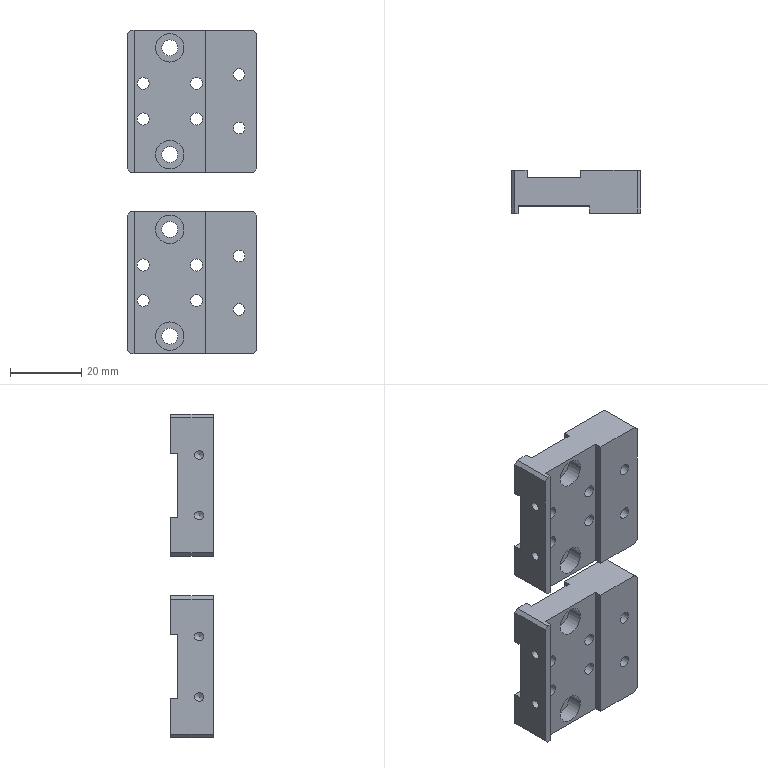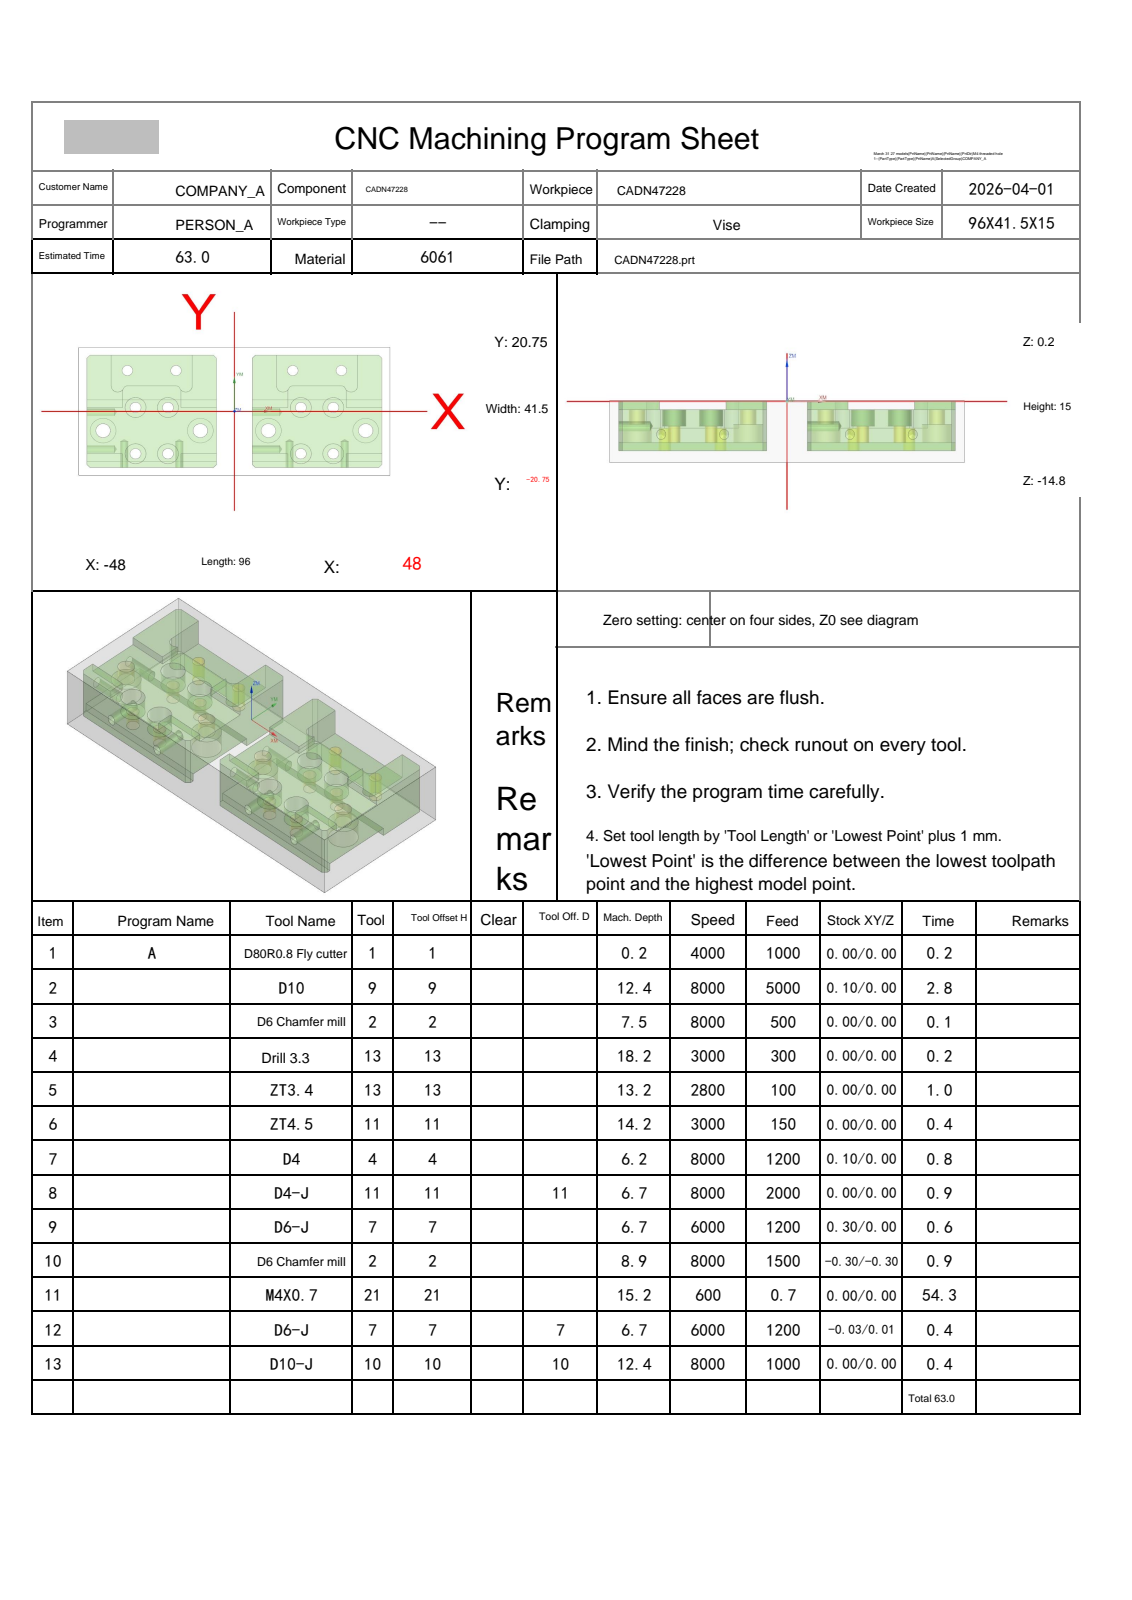NC program | NX | posted by the shop | part box 36.5 x 12 x 91 mm
Lines 1840 to 2876 of 5439:
N8 T11 M06
(D4-J  D=4. R=0. H=11 ce=0.00 di=0.00)
G00 G90 G54 X30.5 Y1.25 M03 S8000
G43 H11 Z20.
M08
Z-1.5
G41 D11
G01 X30.69 Y1.312 F500.
G03 X31.109 Y1.891 I-.19 J.579
X30.5 Y2.5 I-.609 J0.0
X31.235 Y2.261 Z-6. I0.0 J-1.25
X30.5 Y2.5 I-.735 J-1.011
X29.25 Y1.25 I0.0 J-1.25
X30.5 Y0.0 I1.25 J0.0
X31.75 Y1.25 I0.0 J1.25
X31.235 Y2.261 I-1.25 J0.0
X30.877 Y2.378 I-.358 J-.493
X30.268 Y1.769 I0.0 J-.609
X30.383 Y1.412 I.609 J0.0
G01 G40 X30.5 Y1.25
G00 Z20.
X20.5
Z-1.5
G41 D11
G01 X20.69 Y1.312
G03 X21.109 Y1.891 I-.19 J.579
X20.5 Y2.5 I-.609 J0.0
X21.235 Y2.261 Z-6. I0.0 J-1.25
X20.5 Y2.5 I-.735 J-1.011
X19.25 Y1.25 I0.0 J-1.25
X20.5 Y0.0 I1.25 J0.0
X21.75 Y1.25 I0.0 J1.25
X21.235 Y2.261 I-1.25 J0.0
X20.877 Y2.378 I-.358 J-.493
X20.268 Y1.769 I0.0 J-.609
X20.383 Y1.412 I.609 J0.0
G01 G40 X20.5 Y1.25
G00 Z20.
X30.5 Y-13.75
Z-1.5
G41 D11
G01 X30.69 Y-13.688
G03 X31.109 Y-13.109 I-.19 J.579
X30.5 Y-12.5 I-.609 J0.0
X31.235 Y-12.739 Z-6. I0.0 J-1.25
X30.5 Y-12.5 I-.735 J-1.011
X29.25 Y-13.75 I0.0 J-1.25
X30.5 Y-15. I1.25 J0.0
X31.75 Y-13.75 I0.0 J1.25
X31.235 Y-12.739 I-1.25 J0.0
X30.877 Y-12.622 I-.358 J-.493
X30.268 Y-13.231 I0.0 J-.609
X30.383 Y-13.588 I.609 J0.0
G01 G40 X30.5 Y-13.75
G00 Z20.
X20.5
Z-1.5
G41 D11
G01 X20.69 Y-13.688
G03 X21.109 Y-13.109 I-.19 J.579
X20.5 Y-12.5 I-.609 J0.0
X21.235 Y-12.739 Z-6. I0.0 J-1.25
X20.5 Y-12.5 I-.735 J-1.011
X19.25 Y-13.75 I0.0 J-1.25
X20.5 Y-15. I1.25 J0.0
X21.75 Y-13.75 I0.0 J1.25
X21.235 Y-12.739 I-1.25 J0.0
X20.877 Y-12.622 I-.358 J-.493
X20.268 Y-13.231 I0.0 J-.609
X20.383 Y-13.588 I.609 J0.0
G01 G40 X20.5 Y-13.75
G00 Z20.
X-20.5
Z-1.5
G41 D11
G01 X-20.31 Y-13.688
G03 X-19.891 Y-13.109 I-.19 J.579
X-20.5 Y-12.5 I-.609 J0.0
X-19.765 Y-12.739 Z-6. I0.0 J-1.25
X-20.5 Y-12.5 I-.735 J-1.011
X-21.75 Y-13.75 I0.0 J-1.25
X-20.5 Y-15. I1.25 J0.0
X-19.25 Y-13.75 I0.0 J1.25
X-19.765 Y-12.739 I-1.25 J0.0
X-20.123 Y-12.622 I-.358 J-.493
X-20.732 Y-13.231 I0.0 J-.609
X-20.617 Y-13.588 I.609 J0.0
G01 G40 X-20.5 Y-13.75
G00 Z20.
X-30.5
Z-1.5
G41 D11
G01 X-30.31 Y-13.688
G03 X-29.891 Y-13.109 I-.19 J.579
X-30.5 Y-12.5 I-.609 J0.0
X-29.765 Y-12.739 Z-6. I0.0 J-1.25
X-30.5 Y-12.5 I-.735 J-1.011
X-31.75 Y-13.75 I0.0 J-1.25
X-30.5 Y-15. I1.25 J0.0
X-29.25 Y-13.75 I0.0 J1.25
X-29.765 Y-12.739 I-1.25 J0.0
X-30.123 Y-12.622 I-.358 J-.493
X-30.732 Y-13.231 I0.0 J-.609
X-30.617 Y-13.588 I.609 J0.0
G01 G40 X-30.5 Y-13.75
G00 Z20.
Y1.25
Z-1.5
G41 D11
G01 X-30.31 Y1.312
G03 X-29.891 Y1.891 I-.19 J.579
X-30.5 Y2.5 I-.609 J0.0
X-29.765 Y2.261 Z-6. I0.0 J-1.25
X-30.5 Y2.5 I-.735 J-1.011
X-31.75 Y1.25 I0.0 J-1.25
X-30.5 Y0.0 I1.25 J0.0
X-29.25 Y1.25 I0.0 J1.25
X-29.765 Y2.261 I-1.25 J0.0
X-30.123 Y2.378 I-.358 J-.493
X-30.732 Y1.769 I0.0 J-.609
X-30.617 Y1.412 I.609 J0.0
G01 G40 X-30.5 Y1.25
G00 Z20.
X-20.5
Z-1.5
G41 D11
G01 X-20.31 Y1.312
G03 X-19.891 Y1.891 I-.19 J.579
X-20.5 Y2.5 I-.609 J0.0
X-19.765 Y2.261 Z-6. I0.0 J-1.25
X-20.5 Y2.5 I-.735 J-1.011
X-21.75 Y1.25 I0.0 J-1.25
X-20.5 Y0.0 I1.25 J0.0
X-19.25 Y1.25 I0.0 J1.25
X-19.765 Y2.261 I-1.25 J0.0
X-20.123 Y2.378 I-.358 J-.493
X-20.732 Y1.769 I0.0 J-.609
X-20.617 Y1.412 I.609 J0.0
G01 G40 X-20.5 Y1.25
G00 Z20.
G00 G90 X-15. Y8.25 M03 S6000
Z20.
Z.305
G01 Z-.295 F1600.
Y11.85 F2000.
X-15.009 Y11.894 Z-.296
X-15.032 Y11.907 Z-.299
X-15.069 Y11.893 Z-.304
X-15.115 Y11.853 Z-.311
X-15.169 Y11.79 Z-.319
X-15.227 Y11.708 Z-.328
X-15.287 Y11.607 Z-.339
X-15.346 Y11.491 Z-.35
X-15.401 Y11.363 Z-.362
X-15.45 Y11.225 Z-.375
X-15.522 Y10.926 Z-.402
X-15.558 Y10.605 Z-.429
Y10.267 Z-.457
X-15.522 Y9.922 Z-.484
X-15.45 Y9.575 Z-.51
X-15.388 Y9.361 Z-.526
X-15.215 Y8.891 Z-.559
X-15.049 Y8.461 Z-.584
X-15.013 Y8.341 Z-.589
X-15. Y8.25 Z-.59
Y11.85
X-15.009 Y11.894 Z-.592
X-15.032 Y11.907 Z-.595
X-15.069 Y11.893 Z-.6
X-15.115 Y11.853 Z-.606
X-15.169 Y11.79 Z-.614
X-15.227 Y11.708 Z-.624
X-15.287 Y11.607 Z-.634
X-15.346 Y11.491 Z-.646
X-15.401 Y11.363 Z-.658
X-15.45 Y11.225 Z-.67
X-15.522 Y10.926 Z-.697
X-15.558 Y10.605 Z-.724
Y10.267 Z-.752
X-15.522 Y9.922 Z-.779
X-15.45 Y9.575 Z-.806
X-15.388 Y9.361 Z-.822
X-15.215 Y8.891 Z-.854
X-15.049 Y8.461 Z-.879
X-15.013 Y8.341 Z-.884
X-15. Y8.25 Z-.886
Y11.85
X-15.009 Y11.894 Z-.887
X-15.032 Y11.907 Z-.89
X-15.069 Y11.893 Z-.895
X-15.115 Y11.853 Z-.901
X-15.169 Y11.79 Z-.91
X-15.227 Y11.708 Z-.919
X-15.287 Y11.607 Z-.929
X-15.346 Y11.491 Z-.941
X-15.401 Y11.363 Z-.953
X-15.45 Y11.225 Z-.966
X-15.522 Y10.926 Z-.992
X-15.558 Y10.605 Z-1.019
Y10.267 Z-1.047
X-15.522 Y9.922 Z-1.074
X-15.45 Y9.575 Z-1.101
X-15.388 Y9.361 Z-1.117
X-15.215 Y8.891 Z-1.149
X-15.049 Y8.461 Z-1.174
X-15.013 Y8.341 Z-1.179
X-15. Y8.25 Z-1.181
Y11.85
X-15.009 Y11.894 Z-1.182
X-15.032 Y11.907 Z-1.185
X-15.069 Y11.893 Z-1.19
X-15.115 Y11.853 Z-1.197
X-15.169 Y11.79 Z-1.205
X-15.227 Y11.708 Z-1.214
X-15.287 Y11.607 Z-1.225
X-15.346 Y11.491 Z-1.236
X-15.401 Y11.363 Z-1.248
X-15.45 Y11.225 Z-1.261
X-15.522 Y10.926 Z-1.287
X-15.558 Y10.605 Z-1.315
Y10.267 Z-1.342
X-15.522 Y9.922 Z-1.37
X-15.45 Y9.575 Z-1.396
X-15.388 Y9.361 Z-1.412
X-15.215 Y8.891 Z-1.444
X-15.049 Y8.461 Z-1.47
X-15.013 Y8.341 Z-1.474
X-15. Y8.25 Z-1.476
Y11.85
X-15.009 Y11.894 Z-1.477
X-15.032 Y11.907 Z-1.48
X-15.069 Y11.893 Z-1.485
X-15.115 Y11.853 Z-1.492
X-15.169 Y11.79 Z-1.5
X-15.227 Y11.708 Z-1.509
X-15.287 Y11.607 Z-1.52
X-15.346 Y11.491 Z-1.531
X-15.401 Y11.363 Z-1.543
X-15.45 Y11.225 Z-1.556
X-15.522 Y10.926 Z-1.583
X-15.558 Y10.605 Z-1.61
Y10.267 Z-1.638
X-15.522 Y9.922 Z-1.665
X-15.45 Y9.575 Z-1.691
X-15.388 Y9.361 Z-1.707
X-15.215 Y8.891 Z-1.74
X-15.049 Y8.461 Z-1.765
X-15.013 Y8.341 Z-1.77
X-15. Y8.25 Z-1.771
Y11.85
X-15.019 Y11.902 Z-1.772
X-15.075 Y11.938 Z-1.776
X-15.161 Y11.961 Z-1.78
X-15.274 Y11.97 Z-1.787
X-15.41 Y11.968 Z-1.795
X-15.563 Y11.955 Z-1.805
X-15.728 Y11.933 Z-1.815
X-15.993 Y11.883 Z-1.833
X-16.258 Y11.821 Z-1.851
X-16.599 Y11.719 Z-1.878
X-16.917 Y11.595 Z-1.905
X-17.212 Y11.449 Z-1.933
X-17.482 Y11.278 Z-1.96
X-17.726 Y11.079 Z-1.987
X-17.838 Y10.97 Z-1.999
X-17.941 Y10.857 Z-2.011
X-18.033 Y10.744 Z-2.023
X-18.111 Y10.634 Z-2.033
X-18.175 Y10.532 Z-2.043
X-18.22 Y10.44 Z-2.051
X-18.246 Y10.362 Z-2.057
X-18.25 Y10.302 Z-2.062
X-18.231 Y10.264 Z-2.066
X-18.184 Y10.25 Z-2.067
X-17.828
G02 X-15. Y8.25 I0.0 J-3.
G01 Y13.403
X-15.016 Y13.446
X-15.062 Y13.468 Z-2.07
X-15.135 Y13.469 Z-2.074
X-15.23 Y13.452 Z-2.08
X-15.346 Y13.419 Z-2.087
X-15.477 Y13.37 Z-2.095
X-15.622 Y13.307 Z-2.103
X-15.775 Y13.233 Z-2.113
X-15.935 Y13.148 Z-2.124
X-16.097 Y13.054 Z-2.135
X-16.258 Y12.953 Z-2.147
X-16.599 Y12.712 Z-2.173
X-16.917 Y12.445 Z-2.2
X-17.212 Y12.153 Z-2.228
X-17.482 Y11.838 Z-2.255
X-17.726 Y11.5 Z-2.282
X-17.828 Y11.34 Z-2.293
X-17.923 Y11.179 Z-2.305
X-18.009 Y11.02 Z-2.315
X-18.084 Y10.868 Z-2.325
X-18.148 Y10.724 Z-2.334
X-18.198 Y10.594 Z-2.342
X-18.232 Y10.479 Z-2.349
X-18.25 Y10.384 Z-2.354
X-18.249 Y10.312 Z-2.358
X-18.227 Y10.266 Z-2.361
X-18.184 Y10.25 Z-2.362
X-17.828
G02 X-15. Y8.25 I0.0 J-3.
G01 Y13.403
X-15.016 Y13.446 Z-2.363
X-15.062 Y13.468 Z-2.365
X-15.135 Y13.469 Z-2.369
X-15.23 Y13.452 Z-2.375
X-15.346 Y13.419 Z-2.382
X-15.477 Y13.37 Z-2.39
X-15.622 Y13.307 Z-2.399
X-15.775 Y13.233 Z-2.409
X-15.935 Y13.148 Z-2.419
X-16.097 Y13.054 Z-2.43
X-16.258 Y12.953 Z-2.442
X-16.599 Y12.712 Z-2.468
X-16.917 Y12.445 Z-2.496
X-17.212 Y12.153 Z-2.523
X-17.482 Y11.838 Z-2.551
X-17.726 Y11.5 Z-2.577
X-17.828 Y11.34 Z-2.589
X-17.923 Y11.179 Z-2.6
X-18.009 Y11.02 Z-2.61
X-18.084 Y10.868 Z-2.62
X-18.148 Y10.724 Z-2.629
X-18.198 Y10.594 Z-2.637
X-18.232 Y10.479 Z-2.644
X-18.25 Y10.384 Z-2.649
X-18.249 Y10.312 Z-2.654
X-18.227 Y10.266 Z-2.656
X-18.184 Y10.25 Z-2.657
X-17.828
G02 X-15. Y8.25 I0.0 J-3.
G01 Y13.403
X-15.016 Y13.446 Z-2.658
X-15.062 Y13.468 Z-2.661
X-15.135 Y13.469 Z-2.665
X-15.23 Y13.452 Z-2.67
X-15.346 Y13.419 Z-2.677
X-15.477 Y13.37 Z-2.685
X-15.622 Y13.307 Z-2.694
X-15.775 Y13.233 Z-2.704
X-15.935 Y13.148 Z-2.714
X-16.097 Y13.054 Z-2.725
X-16.258 Y12.953 Z-2.737
X-16.599 Y12.712 Z-2.763
X-16.917 Y12.445 Z-2.791
X-17.212 Y12.153 Z-2.818
X-17.482 Y11.838 Z-2.846
X-17.726 Y11.5 Z-2.872
X-17.828 Y11.34 Z-2.884
X-17.923 Y11.179 Z-2.895
X-18.009 Y11.02 Z-2.906
X-18.084 Y10.868 Z-2.915
X-18.148 Y10.724 Z-2.924
X-18.198 Y10.594 Z-2.932
X-18.232 Y10.479 Z-2.939
X-18.25 Y10.384 Z-2.945
X-18.249 Y10.312 Z-2.949
X-18.227 Y10.266 Z-2.951
X-18.184 Y10.25 Z-2.952
X-17.828
G02 X-15. Y8.25 I0.0 J-3.
G01 Y13.403
X-15.016 Y13.446 Z-2.953
X-15.062 Y13.468 Z-2.956
X-15.135 Y13.469 Z-2.96
X-15.23 Y13.452 Z-2.965
X-15.346 Y13.419 Z-2.972
X-15.477 Y13.37 Z-2.98
X-15.622 Y13.307 Z-2.989
X-15.775 Y13.233 Z-2.999
X-15.935 Y13.148 Z-3.01
X-16.097 Y13.054 Z-3.021
X-16.258 Y12.953 Z-3.032
X-16.599 Y12.712 Z-3.059
X-16.917 Y12.445 Z-3.086
X-17.212 Y12.153 Z-3.114
X-17.482 Y11.838 Z-3.141
X-17.726 Y11.5 Z-3.168
X-17.828 Y11.34 Z-3.179
X-17.923 Y11.179 Z-3.19
X-18.009 Y11.02 Z-3.201
X-18.084 Y10.868 Z-3.211
X-18.148 Y10.724 Z-3.22
X-18.198 Y10.594 Z-3.228
X-18.232 Y10.479 Z-3.234
X-18.25 Y10.384 Z-3.24
X-18.249 Y10.312 Z-3.244
X-18.227 Y10.266 Z-3.247
X-18.184 Y10.25 Z-3.248
X-17.828
G02 X-15. Y8.25 I0.0 J-3.
G01 Y13.403
X-15.016 Y13.446
X-15.062 Y13.468 Z-3.251
X-15.135 Y13.469 Z-3.255
X-15.23 Y13.452 Z-3.261
X-15.346 Y13.419 Z-3.267
X-15.477 Y13.37 Z-3.275
X-15.622 Y13.307 Z-3.284
X-15.775 Y13.233 Z-3.294
X-15.935 Y13.148 Z-3.305
X-16.097 Y13.054 Z-3.316
X-16.258 Y12.953 Z-3.327
X-16.599 Y12.712 Z-3.354
X-16.917 Y12.445 Z-3.381
X-17.212 Y12.153 Z-3.409
X-17.482 Y11.838 Z-3.436
X-17.726 Y11.5 Z-3.463
X-17.828 Y11.34 Z-3.474
X-17.923 Y11.179 Z-3.485
X-18.009 Y11.02 Z-3.496
X-18.084 Y10.868 Z-3.506
X-18.148 Y10.724 Z-3.515
X-18.198 Y10.594 Z-3.523
X-18.232 Y10.479 Z-3.53
X-18.25 Y10.384 Z-3.535
X-18.249 Y10.312 Z-3.539
X-18.227 Y10.266 Z-3.542
X-18.184 Y10.25 Z-3.543
X-17.828
G02 X-15. Y8.25 I0.0 J-3.
G01 Y13.403
X-15.016 Y13.446 Z-3.544
X-15.062 Y13.468 Z-3.546
X-15.135 Y13.469 Z-3.55
X-15.23 Y13.452 Z-3.556
X-15.346 Y13.419 Z-3.563
X-15.477 Y13.37 Z-3.571
X-15.622 Y13.307 Z-3.58
X-15.775 Y13.233 Z-3.589
X-15.935 Y13.148 Z-3.6
X-16.097 Y13.054 Z-3.611
X-16.258 Y12.953 Z-3.623
X-16.599 Y12.712 Z-3.649
X-16.917 Y12.445 Z-3.677
X-17.212 Y12.153 Z-3.704
X-17.482 Y11.838 Z-3.732
X-17.726 Y11.5 Z-3.758
X-17.828 Y11.34 Z-3.77
X-17.923 Y11.179 Z-3.781
X-18.009 Y11.02 Z-3.791
X-18.084 Y10.868 Z-3.801
X-18.148 Y10.724 Z-3.81
X-18.198 Y10.594 Z-3.818
X-18.232 Y10.479 Z-3.825
X-18.25 Y10.384 Z-3.83
X-18.249 Y10.312 Z-3.834
X-18.227 Y10.266 Z-3.837
X-18.184 Y10.25 Z-3.838
X-17.828
G02 X-15. Y8.25 I0.0 J-3.
G01 Y13.403
X-15.016 Y13.446 Z-3.839
X-15.062 Y13.468 Z-3.841
X-15.135 Y13.469 Z-3.846
X-15.23 Y13.452 Z-3.851
X-15.346 Y13.419 Z-3.858
X-15.477 Y13.37 Z-3.866
X-15.622 Y13.307 Z-3.875
X-15.775 Y13.233 Z-3.885
X-15.935 Y13.148 Z-3.895
X-16.097 Y13.054 Z-3.906
X-16.258 Y12.953 Z-3.918
X-16.599 Y12.712 Z-3.944
X-16.917 Y12.445 Z-3.972
X-17.212 Y12.153 Z-3.999
X-17.482 Y11.838 Z-4.027
X-17.726 Y11.5 Z-4.053
X-17.828 Y11.34 Z-4.065
X-17.923 Y11.179 Z-4.076
X-18.009 Y11.02 Z-4.086
X-18.084 Y10.868 Z-4.096
X-18.148 Y10.724 Z-4.105
X-18.198 Y10.594 Z-4.113
X-18.232 Y10.479 Z-4.12
X-18.25 Y10.384 Z-4.126
X-18.249 Y10.312 Z-4.13
X-18.227 Y10.266 Z-4.132
X-18.184 Y10.25 Z-4.133
X-17.828
G02 X-15. Y8.25 I0.0 J-3.
G01 Y13.403
X-15.016 Y13.446 Z-4.134
X-15.062 Y13.468 Z-4.137
X-15.135 Y13.469 Z-4.141
X-15.23 Y13.452 Z-4.146
X-15.346 Y13.419 Z-4.153
X-15.477 Y13.37 Z-4.161
X-15.622 Y13.307 Z-4.17
X-15.775 Y13.233 Z-4.18
X-15.935 Y13.148 Z-4.19
X-16.097 Y13.054 Z-4.202
X-16.258 Y12.953 Z-4.213
X-16.599 Y12.712 Z-4.24
X-16.917 Y12.445 Z-4.267
X-17.212 Y12.153 Z-4.295
X-17.482 Y11.838 Z-4.322
X-17.726 Y11.5 Z-4.348
X-17.828 Y11.34 Z-4.36
X-17.923 Y11.179 Z-4.371
X-18.009 Y11.02 Z-4.382
X-18.084 Y10.868 Z-4.392
X-18.148 Y10.724 Z-4.4
X-18.198 Y10.594 Z-4.408
X-18.232 Y10.479 Z-4.415
X-18.25 Y10.384 Z-4.421
X-18.249 Y10.312 Z-4.425
X-18.227 Y10.266 Z-4.428
X-18.184 Y10.25
X-17.828
G02 X-15. Y8.25 I0.0 J-3.
G01 Y13.403
X-15.016 Y13.446 Z-4.429
X-15.062 Y13.468 Z-4.432
X-15.135 Y13.469 Z-4.436
X-15.23 Y13.452 Z-4.442
X-15.346 Y13.419 Z-4.448
X-15.477 Y13.37 Z-4.456
X-15.622 Y13.307 Z-4.465
X-15.775 Y13.233 Z-4.475
X-15.935 Y13.148 Z-4.486
X-16.097 Y13.054 Z-4.497
X-16.258 Y12.953 Z-4.508
X-16.599 Y12.712 Z-4.535
X-16.917 Y12.445 Z-4.562
X-17.212 Y12.153 Z-4.59
X-17.482 Y11.838 Z-4.617
X-17.726 Y11.5 Z-4.644
X-17.828 Y11.34 Z-4.655
X-17.923 Y11.179 Z-4.666
X-18.009 Y11.02 Z-4.677
X-18.084 Y10.868 Z-4.687
X-18.148 Y10.724 Z-4.696
X-18.198 Y10.594 Z-4.704
X-18.232 Y10.479 Z-4.71
X-18.25 Y10.384 Z-4.716
X-18.249 Y10.312 Z-4.72
X-18.227 Y10.266 Z-4.723
X-18.184 Y10.25 Z-4.724
X-17.828
G02 X-15. Y8.25 I0.0 J-3.
G01 Y13.403
X-15.016 Y13.446 Z-4.725
X-15.062 Y13.468 Z-4.727
X-15.135 Y13.469 Z-4.731
X-15.23 Y13.452 Z-4.737
X-15.346 Y13.419 Z-4.744
X-15.477 Y13.37 Z-4.752
X-15.622 Y13.307 Z-4.761
X-15.775 Y13.233 Z-4.77
X-15.935 Y13.148 Z-4.781
X-16.097 Y13.054 Z-4.792
X-16.258 Y12.953 Z-4.804
X-16.599 Y12.712 Z-4.83
X-16.917 Y12.445 Z-4.857
X-17.212 Y12.153 Z-4.885
X-17.482 Y11.838 Z-4.912
X-17.726 Y11.5 Z-4.939
X-17.828 Y11.34 Z-4.95
X-17.923 Y11.179 Z-4.962
X-18.009 Y11.02 Z-4.972
X-18.084 Y10.868 Z-4.982
X-18.148 Y10.724 Z-4.991
X-18.198 Y10.594 Z-4.999
X-18.232 Y10.479 Z-5.006
X-18.25 Y10.384 Z-5.011
X-18.249 Y10.312 Z-5.015
X-18.227 Y10.266 Z-5.018
X-18.184 Y10.25 Z-5.019
X-17.828
G02 X-15. Y8.25 I0.0 J-3.
G01 Y13.403
X-15.016 Y13.446 Z-5.02
X-15.062 Y13.468 Z-5.022
X-15.135 Y13.469 Z-5.026
X-15.23 Y13.452 Z-5.032
X-15.346 Y13.419 Z-5.039
X-15.477 Y13.37 Z-5.047
X-15.622 Y13.307 Z-5.056
X-15.775 Y13.233 Z-5.066
X-15.935 Y13.148 Z-5.076
X-16.097 Y13.054 Z-5.087
X-16.258 Y12.953 Z-5.099
X-16.599 Y12.712 Z-5.125
X-16.917 Y12.445 Z-5.153
X-17.212 Y12.153 Z-5.18
X-17.482 Y11.838 Z-5.208
X-17.726 Y11.5 Z-5.234
X-17.828 Y11.34 Z-5.246
X-17.923 Y11.179 Z-5.257
X-18.009 Y11.02 Z-5.267
X-18.084 Y10.868 Z-5.277
X-18.148 Y10.724 Z-5.286
X-18.198 Y10.594 Z-5.294
X-18.232 Y10.479 Z-5.301
X-18.25 Y10.384 Z-5.306
X-18.249 Y10.312 Z-5.311
X-18.227 Y10.266 Z-5.313
X-18.184 Y10.25 Z-5.314
X-17.828
G02 X-15. Y8.25 I0.0 J-3.
G01 Y13.403
X-15.016 Y13.446 Z-5.315
X-15.062 Y13.468 Z-5.318
X-15.135 Y13.469 Z-5.322
X-15.23 Y13.452 Z-5.327
X-15.346 Y13.419 Z-5.334
X-15.477 Y13.37 Z-5.342
X-15.622 Y13.307 Z-5.351
X-15.775 Y13.233 Z-5.361
X-15.935 Y13.148 Z-5.371
X-16.097 Y13.054 Z-5.382
X-16.258 Y12.953 Z-5.394
X-16.599 Y12.712 Z-5.421
X-16.917 Y12.445 Z-5.448
X-17.212 Y12.153 Z-5.476
X-17.482 Y11.838 Z-5.503
X-17.726 Y11.5 Z-5.529
X-17.828 Y11.34 Z-5.541
X-17.923 Y11.179 Z-5.552
X-18.009 Y11.02 Z-5.563
X-18.084 Y10.868 Z-5.572
X-18.148 Y10.724 Z-5.581
X-18.198 Y10.594 Z-5.589
X-18.232 Y10.479 Z-5.596
X-18.25 Y10.384 Z-5.602
X-18.249 Y10.312 Z-5.606
X-18.227 Y10.266 Z-5.608
X-18.184 Y10.25 Z-5.609
X-17.828
G02 X-15. Y8.25 I0.0 J-3.
G01 Y13.403
X-15.016 Y13.446 Z-5.61
X-15.062 Y13.468 Z-5.613
X-15.135 Y13.469 Z-5.617
X-15.23 Y13.452 Z-5.622
X-15.346 Y13.419 Z-5.629
X-15.477 Y13.37 Z-5.637
X-15.622 Y13.307 Z-5.646
X-15.775 Y13.233 Z-5.656
X-15.935 Y13.148 Z-5.667
X-16.097 Y13.054 Z-5.678
X-16.258 Y12.953 Z-5.689
X-16.599 Y12.712 Z-5.716
X-16.917 Y12.445 Z-5.743
X-17.212 Y12.153 Z-5.771
X-17.482 Y11.838 Z-5.798
X-17.726 Y11.5 Z-5.825
X-17.828 Y11.34 Z-5.836
X-17.923 Y11.179 Z-5.847
X-18.009 Y11.02 Z-5.858
X-18.084 Y10.868 Z-5.868
X-18.148 Y10.724 Z-5.877
X-18.198 Y10.594 Z-5.885
X-18.232 Y10.479 Z-5.891
X-18.25 Y10.384 Z-5.897
X-18.249 Y10.312 Z-5.901
X-18.227 Y10.266 Z-5.904
X-18.184 Y10.25 Z-5.905
X-17.828
G02 X-15. Y8.25 I0.0 J-3.
G01 Y13.403
X-15.016 Y13.446
X-15.062 Y13.468 Z-5.908
X-15.135 Y13.469 Z-5.912
X-15.23 Y13.452 Z-5.918
X-15.346 Y13.419 Z-5.925
X-15.477 Y13.37 Z-5.932
X-15.622 Y13.307 Z-5.941
X-15.775 Y13.233 Z-5.951
X-15.935 Y13.148 Z-5.962
X-16.097 Y13.054 Z-5.973
X-16.258 Y12.953 Z-5.985
X-16.599 Y12.712 Z-6.011
X-16.917 Y12.445 Z-6.038
X-17.212 Y12.153 Z-6.066
X-17.482 Y11.838 Z-6.093
X-17.726 Y11.5 Z-6.12
X-17.828 Y11.34 Z-6.131
X-17.923 Y11.179 Z-6.143
X-18.009 Y11.02 Z-6.153
X-18.084 Y10.868 Z-6.163
X-18.148 Y10.724 Z-6.172
X-18.198 Y10.594 Z-6.18
X-18.232 Y10.479 Z-6.187
X-18.25 Y10.384 Z-6.192
X-18.249 Y10.312 Z-6.196
X-18.227 Y10.266 Z-6.199
X-18.184 Y10.25 Z-6.2
X-17.828
G02 X-15. Y8.25 I0.0 J-3.
G01 Y13.403
X-15.016 Y13.446 Z-6.201
X-15.062 Y13.468 Z-6.203
X-15.135 Y13.469 Z-6.207
X-15.23 Y13.452 Z-6.213
X-15.346 Y13.419 Z-6.22
X-15.477 Y13.37 Z-6.228
X-15.622 Y13.307 Z-6.237
X-15.775 Y13.233 Z-6.247
X-15.935 Y13.148 Z-6.257
X-16.097 Y13.054 Z-6.268
X-16.258 Y12.953 Z-6.28
X-16.599 Y12.712 Z-6.306
X-16.917 Y12.445 Z-6.334
X-17.212 Y12.153 Z-6.361
X-17.482 Y11.838 Z-6.389
X-17.726 Y11.5 Z-6.415
X-17.828 Y11.34 Z-6.427
X-17.923 Y11.179 Z-6.438
X-18.009 Y11.02 Z-6.448
X-18.084 Y10.868 Z-6.458
X-18.148 Y10.724 Z-6.467
X-18.198 Y10.594 Z-6.475
X-18.232 Y10.479 Z-6.482
X-18.25 Y10.384 Z-6.487
X-18.249 Y10.312 Z-6.492
X-18.227 Y10.266 Z-6.494
X-18.184 Y10.25 Z-6.495
X-17.828
G02 X-15. Y8.25 I0.0 J-3.
G01 Y13.403
X-15.007 Y13.46 Z-6.494
X-15.026 Y13.512 Z-6.489
X-15.055 Y13.559 Z-6.481
X-15.094 Y13.601 Z-6.469
X-15.139 Y13.638 Z-6.453
X-15.19 Y13.67 Z-6.432
X-15.244 Y13.699 Z-6.406
X-15.3 Y13.723 Z-6.375
X-15.356 Y13.744 Z-6.338
X-15.41 Y13.761 Z-6.296
X-15.461 Y13.775 Z-6.247
X-15.506 Y13.786 Z-6.191
X-15.545 Y13.794 Z-6.129
X-15.574 Y13.799 Z-6.059
X-15.593 Y13.802 Z-5.981
X-15.6 Y13.803 Z-5.895
G00 Z3.
X-35.396 Y12.25
Z.305
G01 X-35.403 Y12.249 Z.219 F1600.
X-35.422 Y12.246 Z.141
X-35.452 Y12.24 Z.071
X-35.491 Y12.232 Z.009
X-35.536 Y12.222 Z-.047
X-35.587 Y12.208 Z-.096
X-35.642 Y12.191 Z-.139
X-35.698 Y12.17 Z-.175
X-35.754 Y12.145 Z-.206
X-35.809 Y12.117 Z-.232
X-35.86 Y12.084 Z-.253
X-35.906 Y12.047 Z-.269
X-35.944 Y12.006 Z-.281
X-35.974 Y11.959 Z-.289
X-35.993 Y11.907 Z-.294
X-36. Y11.85 Z-.295
Y8.25 F2000.
X-35.987 Y8.341 Z-.297
X-35.951 Y8.461 Z-.302
X-35.784 Y8.891 Z-.327
X-35.612 Y9.361 Z-.359
X-35.549 Y9.575 Z-.375
X-35.477 Y9.922 Z-.402
X-35.44 Y10.267 Z-.429
Y10.605 Z-.457
X-35.476 Y10.926 Z-.484
X-35.548 Y11.225 Z-.51
X-35.597 Y11.363 Z-.523
X-35.653 Y11.491 Z-.535
X-35.712 Y11.607 Z-.547
X-35.772 Y11.708 Z-.557
X-35.83 Y11.79 Z-.567
X-35.884 Y11.853 Z-.575
X-35.931 Y11.893 Z-.581
X-35.967 Y11.907 Z-.586
X-35.991 Y11.894 Z-.589
X-36. Y11.85 Z-.59
Y8.25
X-35.987 Y8.341 Z-.592
X-35.951 Y8.461 Z-.597
X-35.784 Y8.891 Z-.622
X-35.612 Y9.361 Z-.655
X-35.549 Y9.575 Z-.67
X-35.477 Y9.922 Z-.697
X-35.44 Y10.267 Z-.724
Y10.605 Z-.752
X-35.476 Y10.926 Z-.779
X-35.548 Y11.225 Z-.806
X-35.597 Y11.363 Z-.818
X-35.653 Y11.491 Z-.831
X-35.712 Y11.607 Z-.842
X-35.772 Y11.708 Z-.852
X-35.83 Y11.79 Z-.862
X-35.884 Y11.853 Z-.87
X-35.931 Y11.893 Z-.877
X-35.967 Y11.907 Z-.882
X-35.991 Y11.894 Z-.885
X-36. Y11.85 Z-.886
Y8.25
X-35.987 Y8.341 Z-.887
X-35.951 Y8.461 Z-.892
X-35.784 Y8.891 Z-.917
X-35.612 Y9.361 Z-.95
X-35.549 Y9.575 Z-.966
X-35.477 Y9.922 Z-.992
X-35.44 Y10.267 Z-1.019
Y10.605 Z-1.047
X-35.476 Y10.926 Z-1.074
X-35.548 Y11.225 Z-1.101
X-35.597 Y11.363 Z-1.114
X-35.653 Y11.491 Z-1.126
X-35.712 Y11.607 Z-1.137
X-35.772 Y11.708 Z-1.148
X-35.83 Y11.79 Z-1.157
X-35.884 Y11.853 Z-1.165
X-35.931 Y11.893 Z-1.172
X-35.967 Y11.907 Z-1.177
X-35.991 Y11.894 Z-1.18
X-36. Y11.85 Z-1.181
Y8.25
X-35.987 Y8.341 Z-1.183
X-35.951 Y8.461 Z-1.187
X-35.784 Y8.891 Z-1.213
X-35.612 Y9.361 Z-1.245
X-35.549 Y9.575 Z-1.261
X-35.477 Y9.922 Z-1.287
X-35.44 Y10.267 Z-1.315
Y10.605 Z-1.342
X-35.476 Y10.926 Z-1.37
X-35.548 Y11.225 Z-1.396
X-35.597 Y11.363 Z-1.409
X-35.653 Y11.491 Z-1.421
X-35.712 Y11.607 Z-1.432
X-35.772 Y11.708 Z-1.443
X-35.83 Y11.79 Z-1.452
X-35.884 Y11.853 Z-1.46
X-35.931 Y11.893 Z-1.467
X-35.967 Y11.907 Z-1.472
X-35.991 Y11.894 Z-1.475
X-36. Y11.85 Z-1.476
Y8.25
X-35.987 Y8.341 Z-1.478
X-35.951 Y8.461 Z-1.483
X-35.784 Y8.891 Z-1.508
X-35.612 Y9.361 Z-1.54
X-35.549 Y9.575 Z-1.556
X-35.477 Y9.922 Z-1.583
X-35.44 Y10.267 Z-1.61
Y10.605 Z-1.638
X-35.476 Y10.926 Z-1.665
X-35.548 Y11.225 Z-1.691
X-35.597 Y11.363 Z-1.704
X-35.653 Y11.491 Z-1.716
X-35.712 Y11.607 Z-1.728
X-35.772 Y11.708 Z-1.738
X-35.83 Y11.79 Z-1.748
X-35.884 Y11.853 Z-1.756
X-35.931 Y11.893 Z-1.762
X-35.967 Y11.907 Z-1.767
X-35.991 Y11.894 Z-1.77
X-36. Y11.85 Z-1.771
Y8.25
X-35.991 Y8.326 Z-1.772
X-35.968 Y8.432 Z-1.776
X-35.799 Y9.008 Z-1.801
X-35.647 Y9.56 Z-1.828
X-35.549 Y9.999 Z-1.851
X-35.486 Y10.404 Z-1.873
X-35.448 Y10.813 Z-1.896
X-35.435 Y11.219 Z-1.919
X-35.447 Y11.617 Z-1.942
X-35.485 Y12. Z-1.965
X-35.548 Y12.363 Z-1.987
X-35.592 Y12.549 Z-1.998
X-35.642 Y12.725 Z-2.009
X-35.695 Y12.888 Z-2.02
X-35.75 Y13.035 Z-2.03
X-35.804 Y13.164 Z-2.039
X-35.855 Y13.271 Z-2.047
X-35.902 Y13.355 Z-2.053
X-35.942 Y13.413 Z-2.059
X-35.973 Y13.442 Z-2.063
X-35.993 Y13.44 Z-2.066
X-36. Y13.403 Z-2.067
Y8.25
G02 X-33.172 Y10.25 I2.828 J-1.
G01 X-32.816
X-32.773 Y10.266
X-32.752 Y10.312 Z-2.07
X-32.751 Y10.384 Z-2.074
X-32.77 Y10.48 Z-2.08
X-32.805 Y10.594 Z-2.087
X-32.856 Y10.725 Z-2.095
X-32.92 Y10.869 Z-2.103
X-32.996 Y11.022 Z-2.113
X-33.132 Y11.264 Z-2.13
X-33.281 Y11.503 Z-2.147
X-33.525 Y11.841 Z-2.173
X-33.795 Y12.157 Z-2.2
X-34.088 Y12.45 Z-2.228
X-34.405 Y12.717 Z-2.255
X-34.744 Y12.958 Z-2.282
X-34.905 Y13.059 Z-2.293
X-35.066 Y13.152 Z-2.305
X-35.226 Y13.236 Z-2.315
X-35.379 Y13.31 Z-2.325
X-35.523 Y13.372 Z-2.334
X-35.655 Y13.42 Z-2.342
X-35.77 Y13.454 Z-2.349
X-35.865 Y13.47 Z-2.354
X-35.938 Y13.468 Z-2.358
X-35.984 Y13.446 Z-2.361
X-36. Y13.403 Z-2.362
Y8.25
G02 X-33.172 Y10.25 I2.828 J-1.
G01 X-32.816
X-32.773 Y10.266 Z-2.363
X-32.752 Y10.312 Z-2.365
X-32.751 Y10.384 Z-2.369
X-32.77 Y10.48 Z-2.375
X-32.805 Y10.594 Z-2.382
X-32.856 Y10.725 Z-2.39
X-32.92 Y10.869 Z-2.399
X-32.996 Y11.022 Z-2.409
X-33.132 Y11.264 Z-2.425
X-33.281 Y11.503 Z-2.442
X-33.525 Y11.841 Z-2.468
X-33.795 Y12.157 Z-2.496
X-34.088 Y12.45 Z-2.523
X-34.405 Y12.717 Z-2.551
X-34.744 Y12.958 Z-2.577
X-34.905 Y13.059 Z-2.589
X-35.066 Y13.152 Z-2.6
X-35.226 Y13.236 Z-2.61
X-35.379 Y13.31 Z-2.62
X-35.523 Y13.372 Z-2.629
X-35.655 Y13.42 Z-2.637
X-35.77 Y13.454 Z-2.644
X-35.865 Y13.47 Z-2.649
X-35.938 Y13.468 Z-2.654
X-35.984 Y13.446 Z-2.656
X-36. Y13.403 Z-2.657
Y8.25
G02 X-33.172 Y10.25 I2.828 J-1.
G01 X-32.816
X-32.773 Y10.266 Z-2.658
X-32.752 Y10.312 Z-2.661
X-32.751 Y10.384 Z-2.665
X-32.77 Y10.48 Z-2.67
X-32.805 Y10.594 Z-2.677
X-32.856 Y10.725 Z-2.685
X-32.92 Y10.869 Z-2.694
X-32.996 Y11.022 Z-2.704
X-33.132 Y11.264 Z-2.72
X-33.281 Y11.503 Z-2.737
X-33.525 Y11.841 Z-2.763
X-33.795 Y12.157 Z-2.791
X-34.088 Y12.45 Z-2.818
X-34.405 Y12.717 Z-2.846
X-34.744 Y12.958 Z-2.872
X-34.905 Y13.059 Z-2.884
X-35.066 Y13.152 Z-2.895
X-35.226 Y13.236 Z-2.906
X-35.379 Y13.31 Z-2.915
X-35.523 Y13.372 Z-2.924
X-35.655 Y13.42 Z-2.932
X-35.77 Y13.454 Z-2.939
X-35.865 Y13.47 Z-2.945
X-35.938 Y13.468 Z-2.949
X-35.984 Y13.446 Z-2.951
X-36. Y13.403 Z-2.952
Y8.25
G02 X-33.172 Y10.25 I2.828 J-1.
G01 X-32.816
X-32.773 Y10.266 Z-2.953
X-32.752 Y10.312 Z-2.956
X-32.751 Y10.384 Z-2.96
X-32.77 Y10.48 Z-2.965
X-32.805 Y10.594 Z-2.972
X-32.856 Y10.725 Z-2.98
X-32.92 Y10.869 Z-2.989
X-32.996 Y11.022 Z-2.999
X-33.132 Y11.264 Z-3.015
X-33.281 Y11.503 Z-3.032
X-33.525 Y11.841 Z-3.059
X-33.795 Y12.157 Z-3.086
X-34.088 Y12.45 Z-3.114
X-34.405 Y12.717 Z-3.141
X-34.744 Y12.958 Z-3.168
X-34.905 Y13.059 Z-3.179
X-35.066 Y13.152 Z-3.19
X-35.226 Y13.236 Z-3.201
X-35.379 Y13.31 Z-3.211
X-35.523 Y13.372 Z-3.22
X-35.655 Y13.42 Z-3.228
X-35.77 Y13.454 Z-3.234
X-35.865 Y13.47 Z-3.24
X-35.938 Y13.468 Z-3.244
X-35.984 Y13.446 Z-3.247
X-36. Y13.403 Z-3.248
Y8.25
G02 X-33.172 Y10.25 I2.828 J-1.
G01 X-32.816
X-32.773 Y10.266
X-32.752 Y10.312 Z-3.251
X-32.751 Y10.384 Z-3.255
X-32.77 Y10.48 Z-3.261
X-32.805 Y10.594 Z-3.267
X-32.856 Y10.725 Z-3.275
X-32.92 Y10.869 Z-3.284
X-32.996 Y11.022 Z-3.294
X-33.132 Y11.264 Z-3.31
X-33.281 Y11.503 Z-3.327
X-33.525 Y11.841 Z-3.354
X-33.795 Y12.157 Z-3.381
X-34.088 Y12.45 Z-3.409
X-34.405 Y12.717 Z-3.436
X-34.744 Y12.958 Z-3.463
X-34.905 Y13.059 Z-3.474
X-35.066 Y13.152 Z-3.485
X-35.226 Y13.236 Z-3.496
X-35.379 Y13.31 Z-3.506
X-35.523 Y13.372 Z-3.515
X-35.655 Y13.42 Z-3.523
X-35.77 Y13.454 Z-3.53
X-35.865 Y13.47 Z-3.535
X-35.938 Y13.468 Z-3.539
X-35.984 Y13.446 Z-3.542
X-36. Y13.403 Z-3.543
Y8.25
G02 X-33.172 Y10.25 I2.828 J-1.